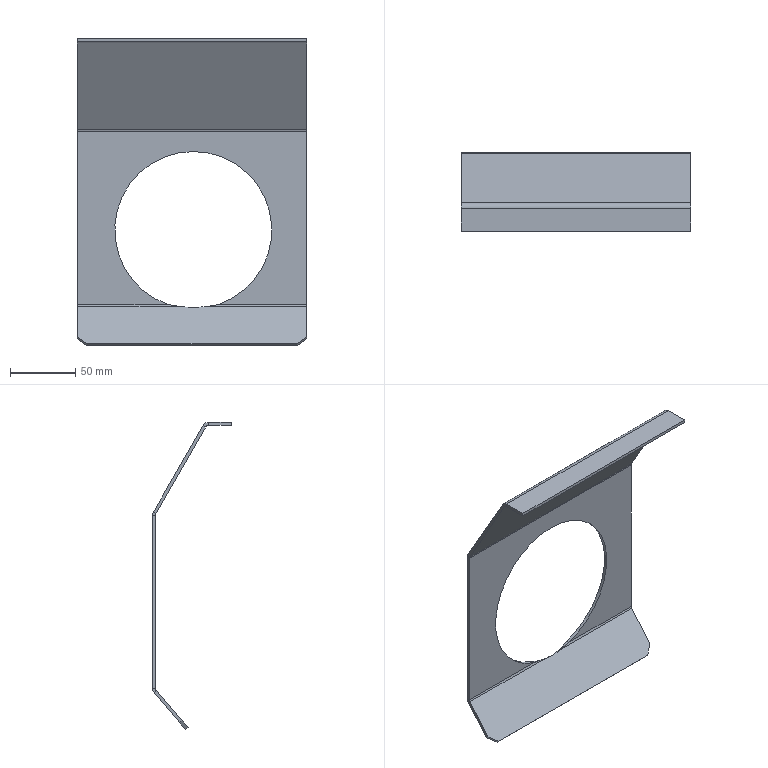Part | SolidWorks | features Chamfer 1, FlatPattern 1, Fold 1, ICE 1, SMBaseFlange 1, SheetMetal 1, UnFold 1 | 1 solid | 39 faces | box 175 x 60.3 x 234.795 mm | volume 83264 mm3 | plane 26 | cylinder 11 | spline 2 | commonest cylinder face diameters 5 x4 9.6 x4 120 x3
STEP:
#1=CARTESIAN_POINT('',(107.594,58.,-201.077));
#2=VERTEX_POINT('',#1);
#3=CARTESIAN_POINT('',(88.5,58.,-84.196));
#4=VERTEX_POINT('',#3);
#5=CARTESIAN_POINT('',(88.5,58.,-144.196));
#6=DIRECTION('',(0.,-1.,0.));
#7=DIRECTION('',(0.,0.,1.));
#8=AXIS2_PLACEMENT_3D('',#5,#6,#7);
#9=CIRCLE('',#8,60.);
#10=EDGE_CURVE('',#2,#4,#9,.T.);
#11=ORIENTED_EDGE('',*,*,#10,.T.);
#12=CARTESIAN_POINT('',(88.5,60.3,-84.196));
#13=VERTEX_POINT('',#12);
#14=CARTESIAN_POINT('',(88.5,57.999,-84.196));
#15=DIRECTION('',(0.,1.,0.));
#16=VECTOR('',#15,1000.);
#17=LINE('',#14,#16);
#18=EDGE_CURVE('',#4,#13,#17,.T.);
#19=ORIENTED_EDGE('',*,*,#18,.T.);
#20=CARTESIAN_POINT('',(107.594,60.3,-201.077));
#21=VERTEX_POINT('',#20);
#22=CARTESIAN_POINT('',(88.5,60.3,-144.196));
#23=DIRECTION('',(0.,1.,0.));
#24=DIRECTION('',(0.,0.,1.));
#25=AXIS2_PLACEMENT_3D('',#22,#23,#24);
#26=CIRCLE('',#25,60.);
#27=EDGE_CURVE('',#13,#21,#26,.T.);
#28=ORIENTED_EDGE('',*,*,#27,.T.);
#29=CARTESIAN_POINT('',(107.594,58.,-201.077));
#30=CARTESIAN_POINT('',(107.594,60.3,-201.077));
#31=B_SPLINE_CURVE_WITH_KNOTS('',1,(#29,#30),.UNSPECIFIED.,.F.,.F.,(2,2),(0.,1.),.UNSPECIFIED.);
#32=EDGE_CURVE('',#2,#21,#31,.T.);
#33=ORIENTED_EDGE('',*,*,#32,.F.);
#34=EDGE_LOOP('',(#11,#19,#28,#33));
#35=FACE_OUTER_BOUND('',#34,.T.);
#36=CARTESIAN_POINT('',(88.5,57.999,-144.196));
#37=DIRECTION('',(0.,1.,0.));
#38=DIRECTION('',(0.,0.,1.));
#39=AXIS2_PLACEMENT_3D('',#36,#37,#38);
#40=CYLINDRICAL_SURFACE('',#39,60.);
#41=ADVANCED_FACE('',(#35),#40,.F.);
#42=CARTESIAN_POINT('',(0.,19.72,-1.256));
#43=VERTEX_POINT('',#42);
#44=CARTESIAN_POINT('',(0.,57.669,-67.422));
#45=VERTEX_POINT('',#44);
#46=CARTESIAN_POINT('',(0.,19.,0.));
#47=DIRECTION('',(0.,0.4975,-0.8675));
#48=VECTOR('',#47,1000.);
#49=LINE('',#46,#48);
#50=EDGE_CURVE('',#43,#45,#49,.T.);
#51=ORIENTED_EDGE('',*,*,#50,.F.);
#52=CARTESIAN_POINT('',(0.,21.716,-0.1119));
#53=VERTEX_POINT('',#52);
#54=CARTESIAN_POINT('',(0.,19.72,-1.256));
#55=DIRECTION('',(0.,0.8675,0.4975));
#56=VECTOR('',#55,1000.);
#57=LINE('',#54,#56);
#58=EDGE_CURVE('',#43,#53,#57,.T.);
#59=ORIENTED_EDGE('',*,*,#58,.T.);
#60=CARTESIAN_POINT('',(0.,59.664,-66.278));
#61=VERTEX_POINT('',#60);
#62=CARTESIAN_POINT('',(0.,20.995,1.144));
#63=DIRECTION('',(0.,0.4975,-0.8675));
#64=VECTOR('',#63,1000.);
#65=LINE('',#62,#64);
#66=EDGE_CURVE('',#53,#61,#65,.T.);
#67=ORIENTED_EDGE('',*,*,#66,.T.);
#68=CARTESIAN_POINT('',(0.,59.664,-66.278));
#69=DIRECTION('',(0.,-0.8675,-0.4975));
#70=VECTOR('',#69,1000.);
#71=LINE('',#68,#70);
#72=EDGE_CURVE('',#61,#45,#71,.T.);
#73=ORIENTED_EDGE('',*,*,#72,.T.);
#74=EDGE_LOOP('',(#51,#59,#67,#73));
#75=FACE_OUTER_BOUND('',#74,.T.);
#76=CARTESIAN_POINT('',(0.,17.552,2.3));
#77=DIRECTION('',(-1.,0.,0.));
#78=DIRECTION('',(0.,0.,1.));
#79=AXIS2_PLACEMENT_3D('',#76,#77,#78);
#80=PLANE('',#79);
#81=ADVANCED_FACE('',(#75),#80,.T.);
#82=CARTESIAN_POINT('',(175.,19.72,-1.256));
#83=VERTEX_POINT('',#82);
#84=CARTESIAN_POINT('',(175.,57.669,-67.422));
#85=VERTEX_POINT('',#84);
#86=CARTESIAN_POINT('',(175.,19.,0.));
#87=DIRECTION('',(0.,0.4975,-0.8675));
#88=VECTOR('',#87,1000.);
#89=LINE('',#86,#88);
#90=EDGE_CURVE('',#83,#85,#89,.T.);
#91=ORIENTED_EDGE('',*,*,#90,.T.);
#92=CARTESIAN_POINT('',(175.,59.664,-66.278));
#93=VERTEX_POINT('',#92);
#94=CARTESIAN_POINT('',(175.,57.669,-67.422));
#95=DIRECTION('',(0.,0.8675,0.4975));
#96=VECTOR('',#95,1000.);
#97=LINE('',#94,#96);
#98=EDGE_CURVE('',#85,#93,#97,.T.);
#99=ORIENTED_EDGE('',*,*,#98,.T.);
#100=CARTESIAN_POINT('',(175.,21.716,-0.1119));
#101=VERTEX_POINT('',#100);
#102=CARTESIAN_POINT('',(175.,20.995,1.144));
#103=DIRECTION('',(0.,0.4975,-0.8675));
#104=VECTOR('',#103,1000.);
#105=LINE('',#102,#104);
#106=EDGE_CURVE('',#101,#93,#105,.T.);
#107=ORIENTED_EDGE('',*,*,#106,.F.);
#108=CARTESIAN_POINT('',(175.,21.716,-0.1119));
#109=DIRECTION('',(0.,-0.8675,-0.4975));
#110=VECTOR('',#109,1000.);
#111=LINE('',#108,#110);
#112=EDGE_CURVE('',#101,#83,#111,.T.);
#113=ORIENTED_EDGE('',*,*,#112,.T.);
#114=EDGE_LOOP('',(#91,#99,#107,#113));
#115=FACE_OUTER_BOUND('',#114,.T.);
#116=CARTESIAN_POINT('',(175.,60.3,-68.666));
#117=DIRECTION('',(1.,0.,0.));
#118=DIRECTION('',(0.,0.,-1.));
#119=AXIS2_PLACEMENT_3D('',#116,#117,#118);
#120=PLANE('',#119);
#121=ADVANCED_FACE('',(#115),#120,.T.);
#122=ORIENTED_EDGE('',*,*,#66,.F.);
#123=CARTESIAN_POINT('',(175.,21.716,-0.1119));
#124=DIRECTION('',(-1.,0.,0.));
#125=VECTOR('',#124,1000.);
#126=LINE('',#123,#125);
#127=EDGE_CURVE('',#101,#53,#126,.T.);
#128=ORIENTED_EDGE('',*,*,#127,.F.);
#129=ORIENTED_EDGE('',*,*,#106,.T.);
#130=CARTESIAN_POINT('',(175.,59.664,-66.278));
#131=DIRECTION('',(-1.,0.,0.));
#132=VECTOR('',#131,1000.);
#133=LINE('',#130,#132);
#134=EDGE_CURVE('',#93,#61,#133,.T.);
#135=ORIENTED_EDGE('',*,*,#134,.T.);
#136=EDGE_LOOP('',(#122,#128,#129,#135));
#137=FACE_OUTER_BOUND('',#136,.T.);
#138=CARTESIAN_POINT('',(175.,20.995,1.144));
#139=DIRECTION('',(0.,0.8675,0.4975));
#140=DIRECTION('',(0.,-0.4975,0.8675));
#141=AXIS2_PLACEMENT_3D('',#138,#139,#140);
#142=PLANE('',#141);
#143=ADVANCED_FACE('',(#137),#142,.T.);
#144=ORIENTED_EDGE('',*,*,#50,.T.);
#145=CARTESIAN_POINT('',(175.,57.669,-67.422));
#146=DIRECTION('',(-1.,0.,0.));
#147=VECTOR('',#146,1000.);
#148=LINE('',#145,#147);
#149=EDGE_CURVE('',#85,#45,#148,.T.);
#150=ORIENTED_EDGE('',*,*,#149,.F.);
#151=ORIENTED_EDGE('',*,*,#90,.F.);
#152=CARTESIAN_POINT('',(175.,19.72,-1.256));
#153=DIRECTION('',(-1.,0.,0.));
#154=VECTOR('',#153,1000.);
#155=LINE('',#152,#154);
#156=EDGE_CURVE('',#83,#43,#155,.T.);
#157=ORIENTED_EDGE('',*,*,#156,.T.);
#158=EDGE_LOOP('',(#144,#150,#151,#157));
#159=FACE_OUTER_BOUND('',#158,.T.);
#160=CARTESIAN_POINT('',(175.,19.,0.));
#161=DIRECTION('',(0.,0.8675,0.4975));
#162=DIRECTION('',(0.,-0.4975,0.8675));
#163=AXIS2_PLACEMENT_3D('',#160,#161,#162);
#164=PLANE('',#163);
#165=ADVANCED_FACE('',(#159),#164,.F.);
#166=CARTESIAN_POINT('',(175.,17.552,0.));
#167=VERTEX_POINT('',#166);
#168=CARTESIAN_POINT('',(175.,17.552,2.3));
#169=VERTEX_POINT('',#168);
#170=CARTESIAN_POINT('',(175.,17.552,0.));
#171=DIRECTION('',(0.,0.,1.));
#172=VECTOR('',#171,1000.);
#173=LINE('',#170,#172);
#174=EDGE_CURVE('',#167,#169,#173,.T.);
#175=ORIENTED_EDGE('',*,*,#174,.F.);
#176=CARTESIAN_POINT('',(175.,17.552,-2.5));
#177=DIRECTION('',(-1.,0.,0.));
#178=DIRECTION('',(0.,0.4975,-0.8675));
#179=AXIS2_PLACEMENT_3D('',#176,#177,#178);
#180=CIRCLE('',#179,2.5);
#181=EDGE_CURVE('',#167,#83,#180,.T.);
#182=ORIENTED_EDGE('',*,*,#181,.T.);
#183=ORIENTED_EDGE('',*,*,#112,.F.);
#184=CARTESIAN_POINT('',(175.,17.552,-2.5));
#185=DIRECTION('',(-1.,0.,0.));
#186=DIRECTION('',(0.,-0.4975,0.8675));
#187=AXIS2_PLACEMENT_3D('',#184,#185,#186);
#188=CIRCLE('',#187,4.8);
#189=EDGE_CURVE('',#169,#101,#188,.T.);
#190=ORIENTED_EDGE('',*,*,#189,.F.);
#191=EDGE_LOOP('',(#175,#182,#183,#190));
#192=FACE_OUTER_BOUND('',#191,.T.);
#193=CARTESIAN_POINT('',(175.,17.552,-2.5));
#194=DIRECTION('',(1.,0.,0.));
#195=DIRECTION('',(0.,0.4975,-0.8675));
#196=AXIS2_PLACEMENT_3D('',#193,#194,#195);
#197=PLANE('',#196);
#198=ADVANCED_FACE('',(#192),#197,.T.);
#199=ORIENTED_EDGE('',*,*,#58,.F.);
#200=CARTESIAN_POINT('',(0.,17.552,0.));
#201=VERTEX_POINT('',#200);
#202=CARTESIAN_POINT('',(0.,17.552,-2.5));
#203=DIRECTION('',(1.,0.,0.));
#204=DIRECTION('',(0.,0.4975,-0.8675));
#205=AXIS2_PLACEMENT_3D('',#202,#203,#204);
#206=CIRCLE('',#205,2.5);
#207=EDGE_CURVE('',#43,#201,#206,.T.);
#208=ORIENTED_EDGE('',*,*,#207,.T.);
#209=CARTESIAN_POINT('',(0.,17.552,2.3));
#210=VERTEX_POINT('',#209);
#211=CARTESIAN_POINT('',(0.,17.552,2.3));
#212=DIRECTION('',(0.,0.,-1.));
#213=VECTOR('',#212,1000.);
#214=LINE('',#211,#213);
#215=EDGE_CURVE('',#210,#201,#214,.T.);
#216=ORIENTED_EDGE('',*,*,#215,.F.);
#217=CARTESIAN_POINT('',(0.,17.552,-2.5));
#218=DIRECTION('',(1.,0.,0.));
#219=DIRECTION('',(0.,0.4975,-0.8675));
#220=AXIS2_PLACEMENT_3D('',#217,#218,#219);
#221=CIRCLE('',#220,4.8);
#222=EDGE_CURVE('',#53,#210,#221,.T.);
#223=ORIENTED_EDGE('',*,*,#222,.F.);
#224=EDGE_LOOP('',(#199,#208,#216,#223));
#225=FACE_OUTER_BOUND('',#224,.T.);
#226=CARTESIAN_POINT('',(0.,17.552,-2.5));
#227=DIRECTION('',(-1.,0.,0.));
#228=DIRECTION('',(0.,-0.4975,0.8675));
#229=AXIS2_PLACEMENT_3D('',#226,#227,#228);
#230=PLANE('',#229);
#231=ADVANCED_FACE('',(#225),#230,.T.);
#232=ORIENTED_EDGE('',*,*,#222,.T.);
#233=CARTESIAN_POINT('',(175.,17.552,2.3));
#234=DIRECTION('',(-1.,0.,0.));
#235=VECTOR('',#234,1000.);
#236=LINE('',#233,#235);
#237=EDGE_CURVE('',#169,#210,#236,.T.);
#238=ORIENTED_EDGE('',*,*,#237,.F.);
#239=ORIENTED_EDGE('',*,*,#189,.T.);
#240=ORIENTED_EDGE('',*,*,#127,.T.);
#241=EDGE_LOOP('',(#232,#238,#239,#240));
#242=FACE_OUTER_BOUND('',#241,.T.);
#243=CARTESIAN_POINT('',(-87.552,17.552,-2.5));
#244=DIRECTION('',(1.,0.,0.));
#245=DIRECTION('',(0.,0.4975,-0.8675));
#246=AXIS2_PLACEMENT_3D('',#243,#244,#245);
#247=CYLINDRICAL_SURFACE('',#246,4.8);
#248=ADVANCED_FACE('',(#242),#247,.T.);
#249=ORIENTED_EDGE('',*,*,#207,.F.);
#250=ORIENTED_EDGE('',*,*,#156,.F.);
#251=ORIENTED_EDGE('',*,*,#181,.F.);
#252=CARTESIAN_POINT('',(175.,17.552,0.));
#253=DIRECTION('',(-1.,0.,0.));
#254=VECTOR('',#253,1000.);
#255=LINE('',#252,#254);
#256=EDGE_CURVE('',#167,#201,#255,.T.);
#257=ORIENTED_EDGE('',*,*,#256,.T.);
#258=EDGE_LOOP('',(#249,#250,#251,#257));
#259=FACE_OUTER_BOUND('',#258,.T.);
#260=CARTESIAN_POINT('',(-87.552,17.552,-2.5));
#261=DIRECTION('',(1.,0.,0.));
#262=DIRECTION('',(0.,0.4975,-0.8675));
#263=AXIS2_PLACEMENT_3D('',#260,#261,#262);
#264=CYLINDRICAL_SURFACE('',#263,2.5);
#265=ADVANCED_FACE('',(#259),#264,.F.);
#266=CARTESIAN_POINT('',(0.,0.,0.));
#267=VERTEX_POINT('',#266);
#268=CARTESIAN_POINT('',(0.,0.,2.3));
#269=VERTEX_POINT('',#268);
#270=CARTESIAN_POINT('',(0.,0.,0.));
#271=DIRECTION('',(0.,0.,1.));
#272=VECTOR('',#271,1000.);
#273=LINE('',#270,#272);
#274=EDGE_CURVE('',#267,#269,#273,.T.);
#275=ORIENTED_EDGE('',*,*,#274,.F.);
#276=CARTESIAN_POINT('',(175.,0.,0.));
#277=VERTEX_POINT('',#276);
#278=CARTESIAN_POINT('',(175.,0.,0.));
#279=DIRECTION('',(-1.,0.,0.));
#280=VECTOR('',#279,1000.);
#281=LINE('',#278,#280);
#282=EDGE_CURVE('',#277,#267,#281,.T.);
#283=ORIENTED_EDGE('',*,*,#282,.F.);
#284=CARTESIAN_POINT('',(175.,0.,2.3));
#285=VERTEX_POINT('',#284);
#286=CARTESIAN_POINT('',(175.,0.,0.));
#287=DIRECTION('',(0.,0.,1.));
#288=VECTOR('',#287,1000.);
#289=LINE('',#286,#288);
#290=EDGE_CURVE('',#277,#285,#289,.T.);
#291=ORIENTED_EDGE('',*,*,#290,.T.);
#292=CARTESIAN_POINT('',(175.,0.,2.3));
#293=DIRECTION('',(-1.,0.,0.));
#294=VECTOR('',#293,1000.);
#295=LINE('',#292,#294);
#296=EDGE_CURVE('',#285,#269,#295,.T.);
#297=ORIENTED_EDGE('',*,*,#296,.T.);
#298=EDGE_LOOP('',(#275,#283,#291,#297));
#299=FACE_OUTER_BOUND('',#298,.T.);
#300=CARTESIAN_POINT('',(175.,0.,0.));
#301=DIRECTION('',(0.,-1.,0.));
#302=DIRECTION('',(0.,0.,-1.));
#303=AXIS2_PLACEMENT_3D('',#300,#301,#302);
#304=PLANE('',#303);
#305=ADVANCED_FACE('',(#299),#304,.T.);
#306=CARTESIAN_POINT('',(0.,0.,2.3));
#307=DIRECTION('',(0.,1.,0.));
#308=VECTOR('',#307,1000.);
#309=LINE('',#306,#308);
#310=EDGE_CURVE('',#269,#210,#309,.T.);
#311=ORIENTED_EDGE('',*,*,#310,.F.);
#312=ORIENTED_EDGE('',*,*,#296,.F.);
#313=CARTESIAN_POINT('',(175.,0.,2.3));
#314=DIRECTION('',(0.,1.,0.));
#315=VECTOR('',#314,1000.);
#316=LINE('',#313,#315);
#317=EDGE_CURVE('',#285,#169,#316,.T.);
#318=ORIENTED_EDGE('',*,*,#317,.T.);
#319=ORIENTED_EDGE('',*,*,#237,.T.);
#320=EDGE_LOOP('',(#311,#312,#318,#319));
#321=FACE_OUTER_BOUND('',#320,.T.);
#322=CARTESIAN_POINT('',(175.,0.,2.3));
#323=DIRECTION('',(0.,0.,1.));
#324=DIRECTION('',(1.,0.,0.));
#325=AXIS2_PLACEMENT_3D('',#322,#323,#324);
#326=PLANE('',#325);
#327=ADVANCED_FACE('',(#321),#326,.T.);
#328=ORIENTED_EDGE('',*,*,#310,.T.);
#329=ORIENTED_EDGE('',*,*,#215,.T.);
#330=CARTESIAN_POINT('',(0.,0.,0.));
#331=DIRECTION('',(0.,1.,0.));
#332=VECTOR('',#331,1000.);
#333=LINE('',#330,#332);
#334=EDGE_CURVE('',#267,#201,#333,.T.);
#335=ORIENTED_EDGE('',*,*,#334,.F.);
#336=ORIENTED_EDGE('',*,*,#274,.T.);
#337=EDGE_LOOP('',(#328,#329,#335,#336));
#338=FACE_OUTER_BOUND('',#337,.T.);
#339=CARTESIAN_POINT('',(0.,55.5,-201.077));
#340=DIRECTION('',(1.,0.,0.));
#341=DIRECTION('',(0.,0.,-1.));
#342=AXIS2_PLACEMENT_3D('',#339,#340,#341);
#343=PLANE('',#342);
#344=ADVANCED_FACE('',(#338),#343,.F.);
#345=ORIENTED_EDGE('',*,*,#334,.T.);
#346=ORIENTED_EDGE('',*,*,#256,.F.);
#347=CARTESIAN_POINT('',(175.,0.,0.));
#348=DIRECTION('',(0.,1.,0.));
#349=VECTOR('',#348,1000.);
#350=LINE('',#347,#349);
#351=EDGE_CURVE('',#277,#167,#350,.T.);
#352=ORIENTED_EDGE('',*,*,#351,.F.);
#353=ORIENTED_EDGE('',*,*,#282,.T.);
#354=EDGE_LOOP('',(#345,#346,#352,#353));
#355=FACE_OUTER_BOUND('',#354,.T.);
#356=CARTESIAN_POINT('',(175.,0.,0.));
#357=DIRECTION('',(0.,0.,1.));
#358=DIRECTION('',(1.,0.,0.));
#359=AXIS2_PLACEMENT_3D('',#356,#357,#358);
#360=PLANE('',#359);
#361=ADVANCED_FACE('',(#355),#360,.F.);
#362=ORIENTED_EDGE('',*,*,#351,.T.);
#363=ORIENTED_EDGE('',*,*,#174,.T.);
#364=ORIENTED_EDGE('',*,*,#317,.F.);
#365=ORIENTED_EDGE('',*,*,#290,.F.);
#366=EDGE_LOOP('',(#362,#363,#364,#365));
#367=FACE_OUTER_BOUND('',#366,.T.);
#368=CARTESIAN_POINT('',(175.,21.716,-0.1119));
#369=DIRECTION('',(1.,0.,0.));
#370=DIRECTION('',(0.,0.,-1.));
#371=AXIS2_PLACEMENT_3D('',#368,#369,#370);
#372=PLANE('',#371);
#373=ADVANCED_FACE('',(#367),#372,.T.);
#374=ORIENTED_EDGE('',*,*,#18,.F.);
#375=CARTESIAN_POINT('',(69.406,58.,-201.077));
#376=VERTEX_POINT('',#375);
#377=CARTESIAN_POINT('',(88.5,58.,-144.196));
#378=DIRECTION('',(0.,-1.,0.));
#379=DIRECTION('',(0.,0.,1.));
#380=AXIS2_PLACEMENT_3D('',#377,#378,#379);
#381=CIRCLE('',#380,60.);
#382=EDGE_CURVE('',#4,#376,#381,.T.);
#383=ORIENTED_EDGE('',*,*,#382,.T.);
#384=CARTESIAN_POINT('',(69.406,60.3,-201.077));
#385=VERTEX_POINT('',#384);
#386=CARTESIAN_POINT('',(69.406,60.3,-201.077));
#387=CARTESIAN_POINT('',(69.406,58.,-201.077));
#388=B_SPLINE_CURVE_WITH_KNOTS('',1,(#386,#387),.UNSPECIFIED.,.F.,.F.,(2,2),(0.,1.),.UNSPECIFIED.);
#389=EDGE_CURVE('',#385,#376,#388,.T.);
#390=ORIENTED_EDGE('',*,*,#389,.F.);
#391=CARTESIAN_POINT('',(88.5,60.3,-144.196));
#392=DIRECTION('',(0.,1.,0.));
#393=DIRECTION('',(0.,0.,1.));
#394=AXIS2_PLACEMENT_3D('',#391,#392,#393);
#395=CIRCLE('',#394,60.);
#396=EDGE_CURVE('',#385,#13,#395,.T.);
#397=ORIENTED_EDGE('',*,*,#396,.T.);
#398=EDGE_LOOP('',(#374,#383,#390,#397));
#399=FACE_OUTER_BOUND('',#398,.T.);
#400=CARTESIAN_POINT('',(88.5,57.999,-144.196));
#401=DIRECTION('',(0.,1.,0.));
#402=DIRECTION('',(0.,0.,1.));
#403=AXIS2_PLACEMENT_3D('',#400,#401,#402);
#404=CYLINDRICAL_SURFACE('',#403,60.);
#405=ADVANCED_FACE('',(#399),#404,.F.);
#406=ORIENTED_EDGE('',*,*,#396,.F.);
#407=CARTESIAN_POINT('',(0.,60.3,-201.077));
#408=VERTEX_POINT('',#407);
#409=CARTESIAN_POINT('',(175.,60.3,-201.077));
#410=DIRECTION('',(-1.,0.,0.));
#411=VECTOR('',#410,1000.);
#412=LINE('',#409,#411);
#413=EDGE_CURVE('',#385,#408,#412,.T.);
#414=ORIENTED_EDGE('',*,*,#413,.T.);
#415=CARTESIAN_POINT('',(0.,60.3,-68.666));
#416=VERTEX_POINT('',#415);
#417=CARTESIAN_POINT('',(0.,60.3,-68.));
#418=DIRECTION('',(0.,0.,-1.));
#419=VECTOR('',#418,1000.);
#420=LINE('',#417,#419);
#421=EDGE_CURVE('',#416,#408,#420,.T.);
#422=ORIENTED_EDGE('',*,*,#421,.F.);
#423=CARTESIAN_POINT('',(175.,60.3,-68.666));
#424=VERTEX_POINT('',#423);
#425=CARTESIAN_POINT('',(175.,60.3,-68.666));
#426=DIRECTION('',(-1.,0.,0.));
#427=VECTOR('',#426,1000.);
#428=LINE('',#425,#427);
#429=EDGE_CURVE('',#424,#416,#428,.T.);
#430=ORIENTED_EDGE('',*,*,#429,.F.);
#431=CARTESIAN_POINT('',(175.,60.3,-201.077));
#432=VERTEX_POINT('',#431);
#433=CARTESIAN_POINT('',(175.,60.3,-68.));
#434=DIRECTION('',(0.,0.,-1.));
#435=VECTOR('',#434,1000.);
#436=LINE('',#433,#435);
#437=EDGE_CURVE('',#424,#432,#436,.T.);
#438=ORIENTED_EDGE('',*,*,#437,.T.);
#439=CARTESIAN_POINT('',(175.,60.3,-201.077));
#440=DIRECTION('',(-1.,0.,0.));
#441=VECTOR('',#440,1000.);
#442=LINE('',#439,#441);
#443=EDGE_CURVE('',#432,#21,#442,.T.);
#444=ORIENTED_EDGE('',*,*,#443,.T.);
#445=ORIENTED_EDGE('',*,*,#27,.F.);
#446=EDGE_LOOP('',(#406,#414,#422,#430,#438,#444,#445));
#447=FACE_OUTER_BOUND('',#446,.T.);
#448=CARTESIAN_POINT('',(175.,60.3,-68.));
#449=DIRECTION('',(0.,1.,0.));
#450=DIRECTION('',(0.,0.,1.));
#451=AXIS2_PLACEMENT_3D('',#448,#449,#450);
#452=PLANE('',#451);
#453=ADVANCED_FACE('',(#447),#452,.T.);
#454=CARTESIAN_POINT('',(175.,58.,-68.666));
#455=VERTEX_POINT('',#454);
#456=CARTESIAN_POINT('',(175.,58.,-201.077));
#457=VERTEX_POINT('',#456);
#458=CARTESIAN_POINT('',(175.,58.,-68.));
#459=DIRECTION('',(0.,0.,-1.));
#460=VECTOR('',#459,1000.);
#461=LINE('',#458,#460);
#462=EDGE_CURVE('',#455,#457,#461,.T.);
#463=ORIENTED_EDGE('',*,*,#462,.T.);
#464=CARTESIAN_POINT('',(175.,58.,-201.077));
#465=DIRECTION('',(0.,1.,0.));
#466=VECTOR('',#465,1000.);
#467=LINE('',#464,#466);
#468=EDGE_CURVE('',#457,#432,#467,.T.);
#469=ORIENTED_EDGE('',*,*,#468,.T.);
#470=ORIENTED_EDGE('',*,*,#437,.F.);
#471=CARTESIAN_POINT('',(175.,60.3,-68.666));
#472=DIRECTION('',(0.,-1.,0.));
#473=VECTOR('',#472,1000.);
#474=LINE('',#471,#473);
#475=EDGE_CURVE('',#424,#455,#474,.T.);
#476=ORIENTED_EDGE('',*,*,#475,.T.);
#477=EDGE_LOOP('',(#463,#469,#470,#476));
#478=FACE_OUTER_BOUND('',#477,.T.);
#479=CARTESIAN_POINT('',(175.,59.148,-204.196));
#480=DIRECTION('',(1.,0.,0.));
#481=DIRECTION('',(0.,0.,-1.));
#482=AXIS2_PLACEMENT_3D('',#479,#480,#481);
#483=PLANE('',#482);
#484=ADVANCED_FACE('',(#478),#483,.T.);
#485=CARTESIAN_POINT('',(0.,58.,-201.077));
#486=VERTEX_POINT('',#485);
#487=CARTESIAN_POINT('',(175.,58.,-201.077));
#488=DIRECTION('',(-1.,0.,0.));
#489=VECTOR('',#488,1000.);
#490=LINE('',#487,#489);
#491=EDGE_CURVE('',#376,#486,#490,.T.);
#492=ORIENTED_EDGE('',*,*,#491,.F.);
#493=ORIENTED_EDGE('',*,*,#382,.F.);
#494=ORIENTED_EDGE('',*,*,#10,.F.);
#495=CARTESIAN_POINT('',(175.,58.,-201.077));
#496=DIRECTION('',(-1.,0.,0.));
#497=VECTOR('',#496,1000.);
#498=LINE('',#495,#497);
#499=EDGE_CURVE('',#457,#2,#498,.T.);
#500=ORIENTED_EDGE('',*,*,#499,.F.);
#501=ORIENTED_EDGE('',*,*,#462,.F.);
#502=CARTESIAN_POINT('',(0.,58.,-68.666));
#503=VERTEX_POINT('',#502);
#504=CARTESIAN_POINT('',(175.,58.,-68.666));
#505=DIRECTION('',(-1.,0.,0.));
#506=VECTOR('',#505,1000.);
#507=LINE('',#504,#506);
#508=EDGE_CURVE('',#455,#503,#507,.T.);
#509=ORIENTED_EDGE('',*,*,#508,.T.);
#510=CARTESIAN_POINT('',(0.,58.,-68.));
#511=DIRECTION('',(0.,0.,-1.));
#512=VECTOR('',#511,1000.);
#513=LINE('',#510,#512);
#514=EDGE_CURVE('',#503,#486,#513,.T.);
#515=ORIENTED_EDGE('',*,*,#514,.T.);
#516=EDGE_LOOP('',(#492,#493,#494,#500,#501,#509,#515));
#517=FACE_OUTER_BOUND('',#516,.T.);
#518=CARTESIAN_POINT('',(175.,58.,-68.));
#519=DIRECTION('',(0.,1.,0.));
#520=DIRECTION('',(0.,0.,1.));
#521=AXIS2_PLACEMENT_3D('',#518,#519,#520);
#522=PLANE('',#521);
#523=ADVANCED_FACE('',(#517),#522,.F.);
#524=ORIENTED_EDGE('',*,*,#514,.F.);
#525=CARTESIAN_POINT('',(0.,58.,-68.666));
#526=DIRECTION('',(0.,1.,0.));
#527=VECTOR('',#526,1000.);
#528=LINE('',#525,#527);
#529=EDGE_CURVE('',#503,#416,#528,.T.);
#530=ORIENTED_EDGE('',*,*,#529,.T.);
#531=ORIENTED_EDGE('',*,*,#421,.T.);
#532=CARTESIAN_POINT('',(0.,60.3,-201.077));
#533=DIRECTION('',(0.,-1.,0.));
#534=VECTOR('',#533,1000.);
#535=LINE('',#532,#534);
#536=EDGE_CURVE('',#408,#486,#535,.T.);
#537=ORIENTED_EDGE('',*,*,#536,.T.);
#538=EDGE_LOOP('',(#524,#530,#531,#537));
#539=FACE_OUTER_BOUND('',#538,.T.);
#540=CARTESIAN_POINT('',(0.,59.664,-66.278));
#541=DIRECTION('',(-1.,0.,0.));
#542=DIRECTION('',(0.,0.,1.));
#543=AXIS2_PLACEMENT_3D('',#540,#541,#542);
#544=PLANE('',#543);
#545=ADVANCED_FACE('',(#539),#544,.T.);
#546=ORIENTED_EDGE('',*,*,#98,.F.);
#547=CARTESIAN_POINT('',(175.,55.5,-68.666));
#548=DIRECTION('',(-1.,0.,0.));
#549=DIRECTION('',(0.,0.,-1.));
#550=AXIS2_PLACEMENT_3D('',#547,#548,#549);
#551=CIRCLE('',#550,2.5);
#552=EDGE_CURVE('',#85,#455,#551,.T.);
#553=ORIENTED_EDGE('',*,*,#552,.T.);
#554=ORIENTED_EDGE('',*,*,#475,.F.);
#555=CARTESIAN_POINT('',(175.,55.5,-68.666));
#556=DIRECTION('',(-1.,0.,0.));
#557=DIRECTION('',(0.,0.,1.));
#558=AXIS2_PLACEMENT_3D('',#555,#556,#557);
#559=CIRCLE('',#558,4.8);
#560=EDGE_CURVE('',#93,#424,#559,.T.);
#561=ORIENTED_EDGE('',*,*,#560,.F.);
#562=EDGE_LOOP('',(#546,#553,#554,#561));
#563=FACE_OUTER_BOUND('',#562,.T.);
#564=CARTESIAN_POINT('',(175.,55.5,-68.666));
#565=DIRECTION('',(1.,0.,0.));
#566=DIRECTION('',(0.,0.,-1.));
#567=AXIS2_PLACEMENT_3D('',#564,#565,#566);
#568=PLANE('',#567);
#569=ADVANCED_FACE('',(#563),#568,.T.);
#570=ORIENTED_EDGE('',*,*,#529,.F.);
#571=CARTESIAN_POINT('',(0.,55.5,-68.666));
#572=DIRECTION('',(1.,0.,0.));
#573=DIRECTION('',(0.,0.,-1.));
#574=AXIS2_PLACEMENT_3D('',#571,#572,#573);
#575=CIRCLE('',#574,2.5);
#576=EDGE_CURVE('',#503,#45,#575,.T.);
#577=ORIENTED_EDGE('',*,*,#576,.T.);
#578=ORIENTED_EDGE('',*,*,#72,.F.);
#579=CARTESIAN_POINT('',(0.,55.5,-68.666));
#580=DIRECTION('',(1.,0.,0.));
#581=DIRECTION('',(0.,0.,-1.));
#582=AXIS2_PLACEMENT_3D('',#579,#580,#581);
#583=CIRCLE('',#582,4.8);
#584=EDGE_CURVE('',#416,#61,#583,.T.);
#585=ORIENTED_EDGE('',*,*,#584,.F.);
#586=EDGE_LOOP('',(#570,#577,#578,#585));
#587=FACE_OUTER_BOUND('',#586,.T.);
#588=CARTESIAN_POINT('',(0.,55.5,-68.666));
#589=DIRECTION('',(-1.,0.,0.));
#590=DIRECTION('',(0.,0.,1.));
#591=AXIS2_PLACEMENT_3D('',#588,#589,#590);
#592=PLANE('',#591);
#593=ADVANCED_FACE('',(#587),#592,.T.);
#594=ORIENTED_EDGE('',*,*,#584,.T.);
#595=ORIENTED_EDGE('',*,*,#134,.F.);
#596=ORIENTED_EDGE('',*,*,#560,.T.);
#597=ORIENTED_EDGE('',*,*,#429,.T.);
#598=EDGE_LOOP('',(#594,#595,#596,#597));
#599=FACE_OUTER_BOUND('',#598,.T.);
#600=CARTESIAN_POINT('',(-87.524,55.5,-68.666));
#601=DIRECTION('',(1.,0.,0.));
#602=DIRECTION('',(0.,0.,-1.));
#603=AXIS2_PLACEMENT_3D('',#600,#601,#602);
#604=CYLINDRICAL_SURFACE('',#603,4.8);
#605=ADVANCED_FACE('',(#599),#604,.T.);
#606=ORIENTED_EDGE('',*,*,#576,.F.);
#607=ORIENTED_EDGE('',*,*,#508,.F.);
#608=ORIENTED_EDGE('',*,*,#552,.F.);
#609=ORIENTED_EDGE('',*,*,#149,.T.);
#610=EDGE_LOOP('',(#606,#607,#608,#609));
#611=FACE_OUTER_BOUND('',#610,.T.);
#612=CARTESIAN_POINT('',(-87.524,55.5,-68.666));
#613=DIRECTION('',(1.,0.,0.));
#614=DIRECTION('',(0.,0.,-1.));
#615=AXIS2_PLACEMENT_3D('',#612,#613,#614);
#616=CYLINDRICAL_SURFACE('',#615,2.5);
#617=ADVANCED_FACE('',(#611),#616,.F.);
#618=ORIENTED_EDGE('',*,*,#389,.T.);
#619=CARTESIAN_POINT('',(79.363,57.4,-202.702));
#620=VERTEX_POINT('',#619);
#621=CARTESIAN_POINT('',(69.406,58.,-201.077));
#622=CARTESIAN_POINT('',(70.285,58.,-201.291));
#623=CARTESIAN_POINT('',(71.132,57.973,-201.483));
#624=CARTESIAN_POINT('',(72.353,57.913,-201.735));
#625=CARTESIAN_POINT('',(72.751,57.89,-201.813));
#626=CARTESIAN_POINT('',(73.337,57.854,-201.92));
#627=CARTESIAN_POINT('',(73.53,57.841,-201.954));
#628=CARTESIAN_POINT('',(73.817,57.822,-202.003));
#629=CARTESIAN_POINT('',(73.912,57.816,-202.019));
#630=CARTESIAN_POINT('',(74.054,57.806,-202.043));
#631=CARTESIAN_POINT('',(74.101,57.803,-202.051));
#632=CARTESIAN_POINT('',(74.171,57.798,-202.062));
#633=CARTESIAN_POINT('',(74.195,57.796,-202.066));
#634=CARTESIAN_POINT('',(74.23,57.794,-202.072));
#635=CARTESIAN_POINT('',(74.242,57.793,-202.073));
#636=CARTESIAN_POINT('',(74.259,57.792,-202.076));
#637=CARTESIAN_POINT('',(74.265,57.791,-202.077));
#638=CARTESIAN_POINT('',(74.277,57.79,-202.079));
#639=CARTESIAN_POINT('',(74.284,57.79,-202.08));
#640=CARTESIAN_POINT('',(75.379,57.713,-202.255));
#641=CARTESIAN_POINT('',(77.07,57.595,-202.474));
#642=CARTESIAN_POINT('',(79.363,57.4,-202.702));
#643=B_SPLINE_CURVE_WITH_KNOTS('',3,(#621,#622,#623,#624,#625,#626,#627,#628,#629,#630,#631,#632,#633,#634,#635,#636,#637,#638,#639,#640,#641,#642),.UNSPECIFIED.,.F.,.F.,(4,2,2,2,2,2,2,2,2,2,4),(0.,0.25,0.375,0.4375,0.4688,0.4844,0.4922,0.4961,0.498,0.5,1.),.UNSPECIFIED.);
#644=EDGE_CURVE('',#376,#620,#643,.T.);
#645=ORIENTED_EDGE('',*,*,#644,.T.);
#646=CARTESIAN_POINT('',(79.363,59.148,-204.196));
#647=VERTEX_POINT('',#646);
#648=CARTESIAN_POINT('',(79.363,57.4,-202.702));
#649=CARTESIAN_POINT('',(79.363,59.148,-204.196));
#650=B_SPLINE_CURVE_WITH_KNOTS('',1,(#648,#649),.UNSPECIFIED.,.F.,.F.,(2,2),(0.,1.),.UNSPECIFIED.);
#651=EDGE_CURVE('',#620,#647,#650,.T.);
#652=ORIENTED_EDGE('',*,*,#651,.T.);
#653=CARTESIAN_POINT('',(69.406,60.3,-201.077));
#654=CARTESIAN_POINT('',(70.285,60.3,-201.488));
#655=CARTESIAN_POINT('',(71.132,60.248,-201.857));
#656=CARTESIAN_POINT('',(72.353,60.134,-202.34));
#657=CARTESIAN_POINT('',(72.751,60.09,-202.489));
#658=CARTESIAN_POINT('',(73.337,60.019,-202.696));
#659=CARTESIAN_POINT('',(73.53,59.995,-202.761));
#660=CARTESIAN_POINT('',(73.817,59.958,-202.856));
#661=CARTESIAN_POINT('',(73.959,59.94,-202.902));
#662=CARTESIAN_POINT('',(74.124,59.918,-202.954));
#663=CARTESIAN_POINT('',(74.206,59.907,-202.98));
#664=CARTESIAN_POINT('',(74.247,59.901,-202.992));
#665=CARTESIAN_POINT('',(74.265,59.899,-202.998));
#666=CARTESIAN_POINT('',(74.277,59.897,-203.001));
#667=CARTESIAN_POINT('',(74.284,59.896,-203.004));
#668=CARTESIAN_POINT('',(74.834,59.822,-203.172));
#669=CARTESIAN_POINT('',(75.529,59.729,-203.359));
#670=CARTESIAN_POINT('',(77.221,59.485,-203.762));
#671=CARTESIAN_POINT('',(78.217,59.335,-203.978));
#672=CARTESIAN_POINT('',(79.363,59.148,-204.196));
#673=B_SPLINE_CURVE_WITH_KNOTS('',3,(#653,#654,#655,#656,#657,#658,#659,#660,#661,#662,#663,#664,#665,#666,#667,#668,#669,#670,#671,#672),.UNSPECIFIED.,.F.,.F.,(4,2,2,2,1,1,1,1,2,2,2,4),(0.,0.25,0.375,0.4375,0.4688,0.4844,0.4922,0.4961,0.498,0.5,0.75,1.),.UNSPECIFIED.);
#674=EDGE_CURVE('',#385,#647,#673,.T.);
#675=ORIENTED_EDGE('',*,*,#674,.F.);
#676=EDGE_LOOP('',(#618,#645,#652,#675));
#677=FACE_OUTER_BOUND('',#676,.T.);
#678=CARTESIAN_POINT('',(69.406,60.3,-201.077));
#679=CARTESIAN_POINT('',(70.285,60.3,-201.488));
#680=CARTESIAN_POINT('',(71.132,60.248,-201.857));
#681=CARTESIAN_POINT('',(72.353,60.134,-202.34));
#682=CARTESIAN_POINT('',(72.751,60.09,-202.489));
#683=CARTESIAN_POINT('',(73.337,60.019,-202.696));
#684=CARTESIAN_POINT('',(73.53,59.995,-202.761));
#685=CARTESIAN_POINT('',(73.817,59.958,-202.856));
#686=CARTESIAN_POINT('',(73.912,59.946,-202.887));
#687=CARTESIAN_POINT('',(74.054,59.927,-202.932));
#688=CARTESIAN_POINT('',(74.101,59.921,-202.947));
#689=CARTESIAN_POINT('',(74.171,59.911,-202.969));
#690=CARTESIAN_POINT('',(74.195,59.908,-202.976));
#691=CARTESIAN_POINT('',(74.23,59.904,-202.987));
#692=CARTESIAN_POINT('',(74.242,59.902,-202.99));
#693=CARTESIAN_POINT('',(74.259,59.9,-202.996));
#694=CARTESIAN_POINT('',(74.265,59.899,-202.998));
#695=CARTESIAN_POINT('',(74.277,59.897,-203.001));
#696=CARTESIAN_POINT('',(74.284,59.896,-203.004));
#697=CARTESIAN_POINT('',(75.379,59.749,-203.339));
#698=CARTESIAN_POINT('',(77.07,59.522,-203.759));
#699=CARTESIAN_POINT('',(79.363,59.148,-204.196));
#700=CARTESIAN_POINT('',(69.406,58.,-201.077));
#701=CARTESIAN_POINT('',(70.285,58.,-201.291));
#702=CARTESIAN_POINT('',(71.132,57.973,-201.483));
#703=CARTESIAN_POINT('',(72.353,57.913,-201.735));
#704=CARTESIAN_POINT('',(72.751,57.89,-201.813));
#705=CARTESIAN_POINT('',(73.337,57.854,-201.92));
#706=CARTESIAN_POINT('',(73.53,57.841,-201.954));
#707=CARTESIAN_POINT('',(73.817,57.822,-202.003));
#708=CARTESIAN_POINT('',(73.912,57.816,-202.019));
#709=CARTESIAN_POINT('',(74.054,57.806,-202.043));
#710=CARTESIAN_POINT('',(74.101,57.803,-202.051));
#711=CARTESIAN_POINT('',(74.171,57.798,-202.062));
#712=CARTESIAN_POINT('',(74.195,57.796,-202.066));
#713=CARTESIAN_POINT('',(74.23,57.794,-202.072));
#714=CARTESIAN_POINT('',(74.242,57.793,-202.073));
#715=CARTESIAN_POINT('',(74.259,57.792,-202.076));
#716=CARTESIAN_POINT('',(74.265,57.791,-202.077));
#717=CARTESIAN_POINT('',(74.277,57.79,-202.079));
#718=CARTESIAN_POINT('',(74.284,57.79,-202.08));
#719=CARTESIAN_POINT('',(75.379,57.713,-202.255));
#720=CARTESIAN_POINT('',(77.07,57.595,-202.474));
#721=CARTESIAN_POINT('',(79.363,57.4,-202.702));
#722=B_SPLINE_SURFACE_WITH_KNOTS('',1,3,((#678,#679,#680,#681,#682,#683,#684,#685,#686,#687,#688,#689,#690,#691,#692,#693,#694,#695,#696,#697,#698,#699),(#700,#701,#702,#703,#704,#705,#706,#707,#708,#709,#710,#711,#712,#713,#714,#715,#716,#717,#718,#719,#720,#721)),.UNSPECIFIED.,.F.,.F.,.F.,(2,2),(4,2,2,2,2,2,2,2,2,2,4),(0.,1.),(0.,0.25,0.375,0.4375,0.4688,0.4844,0.4922,0.4961,0.498,0.5,1.),.UNSPECIFIED.);
#723=ADVANCED_FACE('',(#677),#722,.T.);
#724=CARTESIAN_POINT('',(0.,57.4,-202.702));
#725=VERTEX_POINT('',#724);
#726=CARTESIAN_POINT('',(0.,59.148,-204.196));
#727=VERTEX_POINT('',#726);
#728=CARTESIAN_POINT('',(0.,57.4,-202.702));
#729=DIRECTION('',(0.,0.76,-0.6499));
#730=VECTOR('',#729,1000.);
#731=LINE('',#728,#730);
#732=EDGE_CURVE('',#725,#727,#731,.T.);
#733=ORIENTED_EDGE('',*,*,#732,.F.);
#734=CARTESIAN_POINT('',(0.,55.5,-201.077));
#735=DIRECTION('',(1.,0.,0.));
#736=DIRECTION('',(0.,0.,1.));
#737=AXIS2_PLACEMENT_3D('',#734,#735,#736);
#738=CIRCLE('',#737,2.5);
#739=EDGE_CURVE('',#725,#486,#738,.T.);
#740=ORIENTED_EDGE('',*,*,#739,.T.);
#741=ORIENTED_EDGE('',*,*,#536,.F.);
#742=CARTESIAN_POINT('',(0.,55.5,-201.077));
#743=DIRECTION('',(1.,0.,0.));
#744=DIRECTION('',(0.,0.,-1.));
#745=AXIS2_PLACEMENT_3D('',#742,#743,#744);
#746=CIRCLE('',#745,4.8);
#747=EDGE_CURVE('',#727,#408,#746,.T.);
#748=ORIENTED_EDGE('',*,*,#747,.F.);
#749=EDGE_LOOP('',(#733,#740,#741,#748));
#750=FACE_OUTER_BOUND('',#749,.T.);
#751=CARTESIAN_POINT('',(0.,55.5,-201.077));
#752=DIRECTION('',(-1.,0.,0.));
#753=DIRECTION('',(0.,0.,1.));
#754=AXIS2_PLACEMENT_3D('',#751,#752,#753);
#755=PLANE('',#754);
#756=ADVANCED_FACE('',(#750),#755,.T.);
#757=ORIENTED_EDGE('',*,*,#747,.T.);
#758=ORIENTED_EDGE('',*,*,#413,.F.);
#759=ORIENTED_EDGE('',*,*,#674,.T.);
#760=CARTESIAN_POINT('',(175.,59.148,-204.196));
#761=DIRECTION('',(-1.,0.,0.));
#762=VECTOR('',#761,1000.);
#763=LINE('',#760,#762);
#764=EDGE_CURVE('',#647,#727,#763,.T.);
#765=ORIENTED_EDGE('',*,*,#764,.T.);
#766=EDGE_LOOP('',(#757,#758,#759,#765));
#767=FACE_OUTER_BOUND('',#766,.T.);
#768=CARTESIAN_POINT('',(114.136,55.5,-201.077));
#769=DIRECTION('',(-1.,0.,0.));
#770=DIRECTION('',(0.,0.,1.));
#771=AXIS2_PLACEMENT_3D('',#768,#769,#770);
#772=CYLINDRICAL_SURFACE('',#771,4.8);
#773=ADVANCED_FACE('',(#767),#772,.T.);
#774=ORIENTED_EDGE('',*,*,#739,.F.);
#775=CARTESIAN_POINT('',(175.,57.4,-202.702));
#776=DIRECTION('',(-1.,0.,0.));
#777=VECTOR('',#776,1000.);
#778=LINE('',#775,#777);
#779=EDGE_CURVE('',#620,#725,#778,.T.);
#780=ORIENTED_EDGE('',*,*,#779,.F.);
#781=ORIENTED_EDGE('',*,*,#644,.F.);
#782=ORIENTED_EDGE('',*,*,#491,.T.);
#783=EDGE_LOOP('',(#774,#780,#781,#782));
#784=FACE_OUTER_BOUND('',#783,.T.);
#785=CARTESIAN_POINT('',(114.136,55.5,-201.077));
#786=DIRECTION('',(-1.,0.,0.));
#787=DIRECTION('',(0.,0.,1.));
#788=AXIS2_PLACEMENT_3D('',#785,#786,#787);
#789=CYLINDRICAL_SURFACE('',#788,2.5);
#790=ADVANCED_FACE('',(#784),#789,.F.);
#791=CARTESIAN_POINT('',(97.637,59.148,-204.196));
#792=VERTEX_POINT('',#791);
#793=CARTESIAN_POINT('',(97.637,57.4,-202.702));
#794=VERTEX_POINT('',#793);
#795=CARTESIAN_POINT('',(97.637,59.148,-204.196));
#796=CARTESIAN_POINT('',(97.637,57.4,-202.702));
#797=B_SPLINE_CURVE_WITH_KNOTS('',1,(#795,#796),.UNSPECIFIED.,.F.,.F.,(2,2),(0.,1.),.UNSPECIFIED.);
#798=EDGE_CURVE('',#792,#794,#797,.T.);
#799=ORIENTED_EDGE('',*,*,#798,.T.);
#800=CARTESIAN_POINT('',(97.637,57.4,-202.702));
#801=CARTESIAN_POINT('',(98.532,57.467,-202.624));
#802=CARTESIAN_POINT('',(99.403,57.535,-202.534));
#803=CARTESIAN_POINT('',(100.671,57.635,-202.379));
#804=CARTESIAN_POINT('',(101.088,57.667,-202.324));
#805=CARTESIAN_POINT('',(101.704,57.715,-202.237));
#806=CARTESIAN_POINT('',(101.907,57.73,-202.207));
#807=CARTESIAN_POINT('',(102.21,57.753,-202.16));
#808=CARTESIAN_POINT('',(102.311,57.761,-202.145));
#809=CARTESIAN_POINT('',(102.461,57.772,-202.121));
#810=CARTESIAN_POINT('',(102.512,57.775,-202.113));
#811=CARTESIAN_POINT('',(102.586,57.781,-202.101));
#812=CARTESIAN_POINT('',(102.611,57.783,-202.097));
#813=CARTESIAN_POINT('',(102.649,57.785,-202.09));
#814=CARTESIAN_POINT('',(102.661,57.786,-202.088));
#815=CARTESIAN_POINT('',(102.68,57.788,-202.085));
#816=CARTESIAN_POINT('',(102.686,57.788,-202.084));
#817=CARTESIAN_POINT('',(102.699,57.789,-202.082));
#818=CARTESIAN_POINT('',(102.707,57.789,-202.081));
#819=CARTESIAN_POINT('',(103.201,57.825,-202.));
#820=CARTESIAN_POINT('',(103.853,57.874,-201.879));
#821=CARTESIAN_POINT('',(105.481,57.962,-201.546));
#822=CARTESIAN_POINT('',(106.456,58.,-201.333));
#823=CARTESIAN_POINT('',(107.594,58.,-201.077));
#824=B_SPLINE_CURVE_WITH_KNOTS('',3,(#800,#801,#802,#803,#804,#805,#806,#807,#808,#809,#810,#811,#812,#813,#814,#815,#816,#817,#818,#819,#820,#821,#822,#823),.UNSPECIFIED.,.F.,.F.,(4,2,2,2,2,2,2,2,2,2,2,4),(0.,0.25,0.375,0.4375,0.4688,0.4844,0.4922,0.4961,0.498,0.5,0.75,1.),.UNSPECIFIED.);
#825=EDGE_CURVE('',#794,#2,#824,.T.);
#826=ORIENTED_EDGE('',*,*,#825,.T.);
#827=ORIENTED_EDGE('',*,*,#32,.T.);
#828=CARTESIAN_POINT('',(97.637,59.148,-204.196));
#829=CARTESIAN_POINT('',(98.532,59.276,-204.047));
#830=CARTESIAN_POINT('',(99.403,59.407,-203.875));
#831=CARTESIAN_POINT('',(100.671,59.599,-203.578));
#832=CARTESIAN_POINT('',(101.088,59.661,-203.472));
#833=CARTESIAN_POINT('',(101.704,59.752,-203.304));
#834=CARTESIAN_POINT('',(102.009,59.797,-203.217));
#835=CARTESIAN_POINT('',(102.361,59.847,-203.112));
#836=CARTESIAN_POINT('',(102.537,59.872,-203.058));
#837=CARTESIAN_POINT('',(102.624,59.884,-203.031));
#838=CARTESIAN_POINT('',(102.667,59.89,-203.017));
#839=CARTESIAN_POINT('',(102.689,59.893,-203.01));
#840=CARTESIAN_POINT('',(102.699,59.895,-203.007));
#841=CARTESIAN_POINT('',(102.705,59.896,-203.005));
#842=CARTESIAN_POINT('',(102.709,59.896,-203.004));
#843=CARTESIAN_POINT('',(103.201,59.964,-202.849));
#844=CARTESIAN_POINT('',(103.853,60.058,-202.616));
#845=CARTESIAN_POINT('',(105.481,60.226,-201.977));
#846=CARTESIAN_POINT('',(106.457,60.3,-201.569));
#847=CARTESIAN_POINT('',(107.594,60.3,-201.077));
#848=B_SPLINE_CURVE_WITH_KNOTS('',3,(#828,#829,#830,#831,#832,#833,#834,#835,#836,#837,#838,#839,#840,#841,#842,#843,#844,#845,#846,#847),.UNSPECIFIED.,.F.,.F.,(4,2,2,1,1,1,1,1,1,2,2,2,4),(0.,0.25,0.375,0.4375,0.4688,0.4844,0.4922,0.4961,0.498,0.499,0.5,0.75,1.),.UNSPECIFIED.);
#849=EDGE_CURVE('',#792,#21,#848,.T.);
#850=ORIENTED_EDGE('',*,*,#849,.F.);
#851=EDGE_LOOP('',(#799,#826,#827,#850));
#852=FACE_OUTER_BOUND('',#851,.T.);
#853=CARTESIAN_POINT('',(97.637,59.148,-204.196));
#854=CARTESIAN_POINT('',(98.532,59.276,-204.047));
#855=CARTESIAN_POINT('',(99.403,59.407,-203.875));
#856=CARTESIAN_POINT('',(100.671,59.599,-203.578));
#857=CARTESIAN_POINT('',(101.088,59.661,-203.472));
#858=CARTESIAN_POINT('',(101.704,59.752,-203.304));
#859=CARTESIAN_POINT('',(101.907,59.782,-203.246));
#860=CARTESIAN_POINT('',(102.21,59.826,-203.157));
#861=CARTESIAN_POINT('',(102.311,59.84,-203.127));
#862=CARTESIAN_POINT('',(102.461,59.862,-203.081));
#863=CARTESIAN_POINT('',(102.512,59.869,-203.066));
#864=CARTESIAN_POINT('',(102.586,59.879,-203.043));
#865=CARTESIAN_POINT('',(102.611,59.883,-203.035));
#866=CARTESIAN_POINT('',(102.649,59.888,-203.023));
#867=CARTESIAN_POINT('',(102.661,59.889,-203.019));
#868=CARTESIAN_POINT('',(102.68,59.892,-203.013));
#869=CARTESIAN_POINT('',(102.686,59.893,-203.011));
#870=CARTESIAN_POINT('',(102.699,59.895,-203.007));
#871=CARTESIAN_POINT('',(102.707,59.896,-203.005));
#872=CARTESIAN_POINT('',(103.201,59.964,-202.849));
#873=CARTESIAN_POINT('',(103.853,60.058,-202.616));
#874=CARTESIAN_POINT('',(105.481,60.226,-201.977));
#875=CARTESIAN_POINT('',(106.456,60.3,-201.569));
#876=CARTESIAN_POINT('',(107.594,60.3,-201.077));
#877=CARTESIAN_POINT('',(97.637,57.4,-202.702));
#878=CARTESIAN_POINT('',(98.532,57.467,-202.624));
#879=CARTESIAN_POINT('',(99.403,57.535,-202.534));
#880=CARTESIAN_POINT('',(100.671,57.635,-202.379));
#881=CARTESIAN_POINT('',(101.088,57.667,-202.324));
#882=CARTESIAN_POINT('',(101.704,57.715,-202.237));
#883=CARTESIAN_POINT('',(101.907,57.73,-202.207));
#884=CARTESIAN_POINT('',(102.21,57.753,-202.16));
#885=CARTESIAN_POINT('',(102.311,57.761,-202.145));
#886=CARTESIAN_POINT('',(102.461,57.772,-202.121));
#887=CARTESIAN_POINT('',(102.512,57.775,-202.113));
#888=CARTESIAN_POINT('',(102.586,57.781,-202.101));
#889=CARTESIAN_POINT('',(102.611,57.783,-202.097));
#890=CARTESIAN_POINT('',(102.649,57.785,-202.09));
#891=CARTESIAN_POINT('',(102.661,57.786,-202.088));
#892=CARTESIAN_POINT('',(102.68,57.788,-202.085));
#893=CARTESIAN_POINT('',(102.686,57.788,-202.084));
#894=CARTESIAN_POINT('',(102.699,57.789,-202.082));
#895=CARTESIAN_POINT('',(102.707,57.789,-202.081));
#896=CARTESIAN_POINT('',(103.201,57.825,-202.));
#897=CARTESIAN_POINT('',(103.853,57.874,-201.879));
#898=CARTESIAN_POINT('',(105.481,57.962,-201.546));
#899=CARTESIAN_POINT('',(106.456,58.,-201.333));
#900=CARTESIAN_POINT('',(107.594,58.,-201.077));
#901=B_SPLINE_SURFACE_WITH_KNOTS('',1,3,((#853,#854,#855,#856,#857,#858,#859,#860,#861,#862,#863,#864,#865,#866,#867,#868,#869,#870,#871,#872,#873,#874,#875,#876),(#877,#878,#879,#880,#881,#882,#883,#884,#885,#886,#887,#888,#889,#890,#891,#892,#893,#894,#895,#896,#897,#898,#899,#900)),.UNSPECIFIED.,.F.,.F.,.F.,(2,2),(4,2,2,2,2,2,2,2,2,2,2,4),(0.,1.),(0.,0.25,0.375,0.4375,0.4688,0.4844,0.4922,0.4961,0.498,0.5,0.75,1.),.UNSPECIFIED.);
#902=ADVANCED_FACE('',(#852),#901,.T.);
#903=ORIENTED_EDGE('',*,*,#468,.F.);
#904=CARTESIAN_POINT('',(175.,57.4,-202.702));
#905=VERTEX_POINT('',#904);
#906=CARTESIAN_POINT('',(175.,55.5,-201.077));
#907=DIRECTION('',(-1.,0.,0.));
#908=DIRECTION('',(0.,0.,1.));
#909=AXIS2_PLACEMENT_3D('',#906,#907,#908);
#910=CIRCLE('',#909,2.5);
#911=EDGE_CURVE('',#457,#905,#910,.T.);
#912=ORIENTED_EDGE('',*,*,#911,.T.);
#913=CARTESIAN_POINT('',(175.,59.148,-204.196));
#914=VERTEX_POINT('',#913);
#915=CARTESIAN_POINT('',(175.,59.148,-204.196));
#916=DIRECTION('',(0.,-0.76,0.6499));
#917=VECTOR('',#916,1000.);
#918=LINE('',#915,#917);
#919=EDGE_CURVE('',#914,#905,#918,.T.);
#920=ORIENTED_EDGE('',*,*,#919,.F.);
#921=CARTESIAN_POINT('',(175.,55.5,-201.077));
#922=DIRECTION('',(-1.,0.,0.));
#923=DIRECTION('',(0.,0.,1.));
#924=AXIS2_PLACEMENT_3D('',#921,#922,#923);
#925=CIRCLE('',#924,4.8);
#926=EDGE_CURVE('',#432,#914,#925,.T.);
#927=ORIENTED_EDGE('',*,*,#926,.F.);
#928=EDGE_LOOP('',(#903,#912,#920,#927));
#929=FACE_OUTER_BOUND('',#928,.T.);
#930=CARTESIAN_POINT('',(175.,55.5,-201.077));
#931=DIRECTION('',(1.,0.,0.));
#932=DIRECTION('',(0.,0.,-1.));
#933=AXIS2_PLACEMENT_3D('',#930,#931,#932);
#934=PLANE('',#933);
#935=ADVANCED_FACE('',(#929),#934,.T.);
#936=ORIENTED_EDGE('',*,*,#926,.T.);
#937=CARTESIAN_POINT('',(175.,59.148,-204.196));
#938=DIRECTION('',(-1.,0.,0.));
#939=VECTOR('',#938,1000.);
#940=LINE('',#937,#939);
#941=EDGE_CURVE('',#914,#792,#940,.T.);
#942=ORIENTED_EDGE('',*,*,#941,.T.);
#943=ORIENTED_EDGE('',*,*,#849,.T.);
#944=ORIENTED_EDGE('',*,*,#443,.F.);
#945=EDGE_LOOP('',(#936,#942,#943,#944));
#946=FACE_OUTER_BOUND('',#945,.T.);
#947=CARTESIAN_POINT('',(218.732,55.5,-201.077));
#948=DIRECTION('',(-1.,0.,0.));
#949=DIRECTION('',(0.,0.,1.));
#950=AXIS2_PLACEMENT_3D('',#947,#948,#949);
#951=CYLINDRICAL_SURFACE('',#950,4.8);
#952=ADVANCED_FACE('',(#946),#951,.T.);
#953=ORIENTED_EDGE('',*,*,#911,.F.);
#954=ORIENTED_EDGE('',*,*,#499,.T.);
#955=ORIENTED_EDGE('',*,*,#825,.F.);
#956=CARTESIAN_POINT('',(175.,57.4,-202.702));
#957=DIRECTION('',(-1.,0.,0.));
#958=VECTOR('',#957,1000.);
#959=LINE('',#956,#958);
#960=EDGE_CURVE('',#905,#794,#959,.T.);
#961=ORIENTED_EDGE('',*,*,#960,.F.);
#962=EDGE_LOOP('',(#953,#954,#955,#961));
#963=FACE_OUTER_BOUND('',#962,.T.);
#964=CARTESIAN_POINT('',(218.732,55.5,-201.077));
#965=DIRECTION('',(-1.,0.,0.));
#966=DIRECTION('',(0.,0.,1.));
#967=AXIS2_PLACEMENT_3D('',#964,#965,#966);
#968=CYLINDRICAL_SURFACE('',#967,2.5);
#969=ADVANCED_FACE('',(#963),#968,.F.);
#970=CARTESIAN_POINT('',(168.,33.2,-231.));
#971=VERTEX_POINT('',#970);
#972=CARTESIAN_POINT('',(7.,33.2,-231.));
#973=VERTEX_POINT('',#972);
#974=CARTESIAN_POINT('',(175.,33.2,-231.));
#975=DIRECTION('',(-1.,0.,0.));
#976=VECTOR('',#975,1000.);
#977=LINE('',#974,#976);
#978=EDGE_CURVE('',#971,#973,#977,.T.);
#979=ORIENTED_EDGE('',*,*,#978,.T.);
#980=CARTESIAN_POINT('',(7.,34.948,-232.495));
#981=VERTEX_POINT('',#980);
#982=CARTESIAN_POINT('',(7.,34.948,-232.495));
#983=DIRECTION('',(0.,0.76,-0.6499));
#984=VECTOR('',#983,1000.);
#985=LINE('',#982,#984);
#986=EDGE_CURVE('',#973,#981,#985,.T.);
#987=ORIENTED_EDGE('',*,*,#986,.T.);
#988=CARTESIAN_POINT('',(168.,34.948,-232.495));
#989=VERTEX_POINT('',#988);
#990=CARTESIAN_POINT('',(175.,34.948,-232.495));
#991=DIRECTION('',(-1.,0.,0.));
#992=VECTOR('',#991,1000.);
#993=LINE('',#990,#992);
#994=EDGE_CURVE('',#989,#981,#993,.T.);
#995=ORIENTED_EDGE('',*,*,#994,.F.);
#996=CARTESIAN_POINT('',(168.,34.948,-232.495));
#997=DIRECTION('',(0.,-0.76,0.6499));
#998=VECTOR('',#997,1000.);
#999=LINE('',#996,#998);
#1000=EDGE_CURVE('',#989,#971,#999,.T.);
#1001=ORIENTED_EDGE('',*,*,#1000,.T.);
#1002=EDGE_LOOP('',(#979,#987,#995,#1001));
#1003=FACE_OUTER_BOUND('',#1002,.T.);
#1004=CARTESIAN_POINT('',(175.,34.948,-232.495));
#1005=DIRECTION('',(0.,-0.6499,-0.76));
#1006=DIRECTION('',(0.,0.76,-0.6499));
#1007=AXIS2_PLACEMENT_3D('',#1004,#1005,#1006);
#1008=PLANE('',#1007);
#1009=ADVANCED_FACE('',(#1003),#1008,.T.);
#1010=ORIENTED_EDGE('',*,*,#994,.T.);
#1011=CARTESIAN_POINT('',(0.,39.497,-227.175));
#1012=VERTEX_POINT('',#1011);
#1013=CARTESIAN_POINT('',(71.921,-7.246,-281.835));
#1014=DIRECTION('',(-0.7071,0.4596,0.5374));
#1015=VECTOR('',#1014,1000.);
#1016=LINE('',#1013,#1015);
#1017=EDGE_CURVE('',#981,#1012,#1016,.T.);
#1018=ORIENTED_EDGE('',*,*,#1017,.T.);
#1019=CARTESIAN_POINT('',(0.,59.748,-203.495));
#1020=DIRECTION('',(0.,-0.6499,-0.76));
#1021=VECTOR('',#1020,1000.);
#1022=LINE('',#1019,#1021);
#1023=EDGE_CURVE('',#727,#1012,#1022,.T.);
#1024=ORIENTED_EDGE('',*,*,#1023,.F.);
#1025=ORIENTED_EDGE('',*,*,#764,.F.);
#1026=CARTESIAN_POINT('',(88.5,97.689,-159.129));
#1027=DIRECTION('',(0.,0.76,-0.6499));
#1028=DIRECTION('',(0.,0.6499,0.76));
#1029=AXIS2_PLACEMENT_3D('',#1026,#1027,#1028);
#1030=CIRCLE('',#1029,60.);
#1031=EDGE_CURVE('',#792,#647,#1030,.T.);
#1032=ORIENTED_EDGE('',*,*,#1031,.F.);
#1033=ORIENTED_EDGE('',*,*,#941,.F.);
#1034=CARTESIAN_POINT('',(175.,39.497,-227.175));
#1035=VERTEX_POINT('',#1034);
#1036=CARTESIAN_POINT('',(175.,59.748,-203.495));
#1037=DIRECTION('',(0.,-0.6499,-0.76));
#1038=VECTOR('',#1037,1000.);
#1039=LINE('',#1036,#1038);
#1040=EDGE_CURVE('',#914,#1035,#1039,.T.);
#1041=ORIENTED_EDGE('',*,*,#1040,.T.);
#1042=CARTESIAN_POINT('',(190.579,49.623,-215.335));
#1043=DIRECTION('',(-0.7071,-0.4596,-0.5374));
#1044=VECTOR('',#1043,1000.);
#1045=LINE('',#1042,#1044);
#1046=EDGE_CURVE('',#1035,#989,#1045,.T.);
#1047=ORIENTED_EDGE('',*,*,#1046,.T.);
#1048=EDGE_LOOP('',(#1010,#1018,#1024,#1025,#1032,#1033,#1041,#1047));
#1049=FACE_OUTER_BOUND('',#1048,.T.);
#1050=CARTESIAN_POINT('',(175.,59.748,-203.495));
#1051=DIRECTION('',(0.,0.76,-0.6499));
#1052=DIRECTION('',(0.,0.6499,0.76));
#1053=AXIS2_PLACEMENT_3D('',#1050,#1051,#1052);
#1054=PLANE('',#1053);
#1055=ADVANCED_FACE('',(#1049),#1054,.T.);
#1056=CARTESIAN_POINT('',(175.,37.749,-225.68));
#1057=VERTEX_POINT('',#1056);
#1058=CARTESIAN_POINT('',(175.,58.,-202.));
#1059=DIRECTION('',(0.,-0.6499,-0.76));
#1060=VECTOR('',#1059,1000.);
#1061=LINE('',#1058,#1060);
#1062=EDGE_CURVE('',#905,#1057,#1061,.T.);
#1063=ORIENTED_EDGE('',*,*,#1062,.T.);
#1064=CARTESIAN_POINT('',(175.,35.85,-224.055));
#1065=DIRECTION('',(0.,0.76,-0.6499));
#1066=VECTOR('',#1065,1000.);
#1067=LINE('',#1064,#1066);
#1068=EDGE_CURVE('',#1057,#1035,#1067,.T.);
#1069=ORIENTED_EDGE('',*,*,#1068,.T.);
#1070=ORIENTED_EDGE('',*,*,#1040,.F.);
#1071=ORIENTED_EDGE('',*,*,#919,.T.);
#1072=EDGE_LOOP('',(#1063,#1069,#1070,#1071));
#1073=FACE_OUTER_BOUND('',#1072,.T.);
#1074=CARTESIAN_POINT('',(175.,55.5,-201.077));
#1075=DIRECTION('',(1.,0.,0.));
#1076=DIRECTION('',(0.,0.,-1.));
#1077=AXIS2_PLACEMENT_3D('',#1074,#1075,#1076);
#1078=PLANE('',#1077);
#1079=ADVANCED_FACE('',(#1073),#1078,.T.);
#1080=CARTESIAN_POINT('',(0.,37.749,-225.68));
#1081=VERTEX_POINT('',#1080);
#1082=CARTESIAN_POINT('',(0.,58.,-202.));
#1083=DIRECTION('',(0.,-0.6499,-0.76));
#1084=VECTOR('',#1083,1000.);
#1085=LINE('',#1082,#1084);
#1086=EDGE_CURVE('',#725,#1081,#1085,.T.);
#1087=ORIENTED_EDGE('',*,*,#1086,.T.);
#1088=CARTESIAN_POINT('',(0.,37.749,-225.68));
#1089=DIRECTION('',(0.7071,-0.4596,-0.5374));
#1090=VECTOR('',#1089,1000.);
#1091=LINE('',#1088,#1090);
#1092=EDGE_CURVE('',#1081,#973,#1091,.T.);
#1093=ORIENTED_EDGE('',*,*,#1092,.T.);
#1094=ORIENTED_EDGE('',*,*,#978,.F.);
#1095=CARTESIAN_POINT('',(168.,33.2,-231.));
#1096=DIRECTION('',(0.7071,0.4596,0.5374));
#1097=VECTOR('',#1096,1000.);
#1098=LINE('',#1095,#1097);
#1099=EDGE_CURVE('',#971,#1057,#1098,.T.);
#1100=ORIENTED_EDGE('',*,*,#1099,.T.);
#1101=ORIENTED_EDGE('',*,*,#1062,.F.);
#1102=ORIENTED_EDGE('',*,*,#960,.T.);
#1103=CARTESIAN_POINT('',(88.5,95.941,-157.634));
#1104=DIRECTION('',(0.,-0.76,0.6499));
#1105=DIRECTION('',(0.,0.6499,0.76));
#1106=AXIS2_PLACEMENT_3D('',#1103,#1104,#1105);
#1107=CIRCLE('',#1106,60.);
#1108=EDGE_CURVE('',#620,#794,#1107,.T.);
#1109=ORIENTED_EDGE('',*,*,#1108,.F.);
#1110=ORIENTED_EDGE('',*,*,#779,.T.);
#1111=EDGE_LOOP('',(#1087,#1093,#1094,#1100,#1101,#1102,#1109,#1110));
#1112=FACE_OUTER_BOUND('',#1111,.T.);
#1113=CARTESIAN_POINT('',(175.,58.,-202.));
#1114=DIRECTION('',(0.,0.76,-0.6499));
#1115=DIRECTION('',(0.,0.6499,0.76));
#1116=AXIS2_PLACEMENT_3D('',#1113,#1114,#1115);
#1117=PLANE('',#1116);
#1118=ADVANCED_FACE('',(#1112),#1117,.F.);
#1119=ORIENTED_EDGE('',*,*,#798,.F.);
#1120=ORIENTED_EDGE('',*,*,#1031,.T.);
#1121=ORIENTED_EDGE('',*,*,#651,.F.);
#1122=ORIENTED_EDGE('',*,*,#1108,.T.);
#1123=EDGE_LOOP('',(#1119,#1120,#1121,#1122));
#1124=FACE_OUTER_BOUND('',#1123,.T.);
#1125=CARTESIAN_POINT('',(88.5,95.94,-157.633));
#1126=DIRECTION('',(0.,0.76,-0.6499));
#1127=DIRECTION('',(0.,0.6499,0.76));
#1128=AXIS2_PLACEMENT_3D('',#1125,#1126,#1127);
#1129=CYLINDRICAL_SURFACE('',#1128,60.);
#1130=ADVANCED_FACE('',(#1124),#1129,.F.);
#1131=ORIENTED_EDGE('',*,*,#1023,.T.);
#1132=CARTESIAN_POINT('',(0.,38.622,-226.426));
#1133=DIRECTION('',(0.,-0.76,0.6499));
#1134=VECTOR('',#1133,1000.);
#1135=LINE('',#1132,#1134);
#1136=EDGE_CURVE('',#1012,#1081,#1135,.T.);
#1137=ORIENTED_EDGE('',*,*,#1136,.T.);
#1138=ORIENTED_EDGE('',*,*,#1086,.F.);
#1139=ORIENTED_EDGE('',*,*,#732,.T.);
#1140=EDGE_LOOP('',(#1131,#1137,#1138,#1139));
#1141=FACE_OUTER_BOUND('',#1140,.T.);
#1142=CARTESIAN_POINT('',(0.,60.3,-201.077));
#1143=DIRECTION('',(-1.,0.,0.));
#1144=DIRECTION('',(0.,0.,1.));
#1145=AXIS2_PLACEMENT_3D('',#1142,#1143,#1144);
#1146=PLANE('',#1145);
#1147=ADVANCED_FACE('',(#1141),#1146,.T.);
#1148=ORIENTED_EDGE('',*,*,#1017,.F.);
#1149=ORIENTED_EDGE('',*,*,#986,.F.);
#1150=ORIENTED_EDGE('',*,*,#1092,.F.);
#1151=ORIENTED_EDGE('',*,*,#1136,.F.);
#1152=EDGE_LOOP('',(#1148,#1149,#1150,#1151));
#1153=FACE_OUTER_BOUND('',#1152,.T.);
#1154=CARTESIAN_POINT('',(0.,38.622,-226.426));
#1155=DIRECTION('',(0.7071,0.4596,0.5374));
#1156=DIRECTION('',(0.,-0.76,0.6499));
#1157=AXIS2_PLACEMENT_3D('',#1154,#1155,#1156);
#1158=PLANE('',#1157);
#1159=ADVANCED_FACE('',(#1153),#1158,.F.);
#1160=ORIENTED_EDGE('',*,*,#1046,.F.);
#1161=ORIENTED_EDGE('',*,*,#1068,.F.);
#1162=ORIENTED_EDGE('',*,*,#1099,.F.);
#1163=ORIENTED_EDGE('',*,*,#1000,.F.);
#1164=EDGE_LOOP('',(#1160,#1161,#1162,#1163));
#1165=FACE_OUTER_BOUND('',#1164,.T.);
#1166=CARTESIAN_POINT('',(168.,34.948,-232.495));
#1167=DIRECTION('',(-0.7071,0.4596,0.5374));
#1168=DIRECTION('',(0.,-0.76,0.6499));
#1169=AXIS2_PLACEMENT_3D('',#1166,#1167,#1168);
#1170=PLANE('',#1169);
#1171=ADVANCED_FACE('',(#1165),#1170,.F.);
#1172=CLOSED_SHELL('',(#41,#81,#121,#143,#165,#198,#231,#248,#265,#305,#327,#344,#361,#373,#405,#453,#484,#523,#545,#569,#593,#605,#617,#723,#756,#773,#790,#902,#935,#952,#969,#1009,#1055,#1079,#1118,#1130,#1147,#1159,#1171));
#1173=MANIFOLD_SOLID_BREP('',#1172);
#1174=CARTESIAN_POINT('',(0.,0.,0.));
#1175=DIRECTION('',(0.,0.,1.));
#1176=DIRECTION('',(1.,0.,0.));
#1177=AXIS2_PLACEMENT_3D('',#1174,#1175,#1176);
#1178=(LENGTH_UNIT()NAMED_UNIT(*)SI_UNIT(.MILLI.,.METRE.));
#1179=UNCERTAINTY_MEASURE_WITH_UNIT(LENGTH_MEASURE(0.00001),#1178,'','');
#1180=(NAMED_UNIT(*)PLANE_ANGLE_UNIT()SI_UNIT($,.RADIAN.));
#1181=(NAMED_UNIT(*)SI_UNIT($,.STERADIAN.)SOLID_ANGLE_UNIT());
#1182=(GEOMETRIC_REPRESENTATION_CONTEXT(3)GLOBAL_UNCERTAINTY_ASSIGNED_CONTEXT((#1179))GLOBAL_UNIT_ASSIGNED_CONTEXT((#1178,#1180,#1181))REPRESENTATION_CONTEXT('',''));
#1183=ADVANCED_BREP_SHAPE_REPRESENTATION('',(#1173,#1177),#1182);